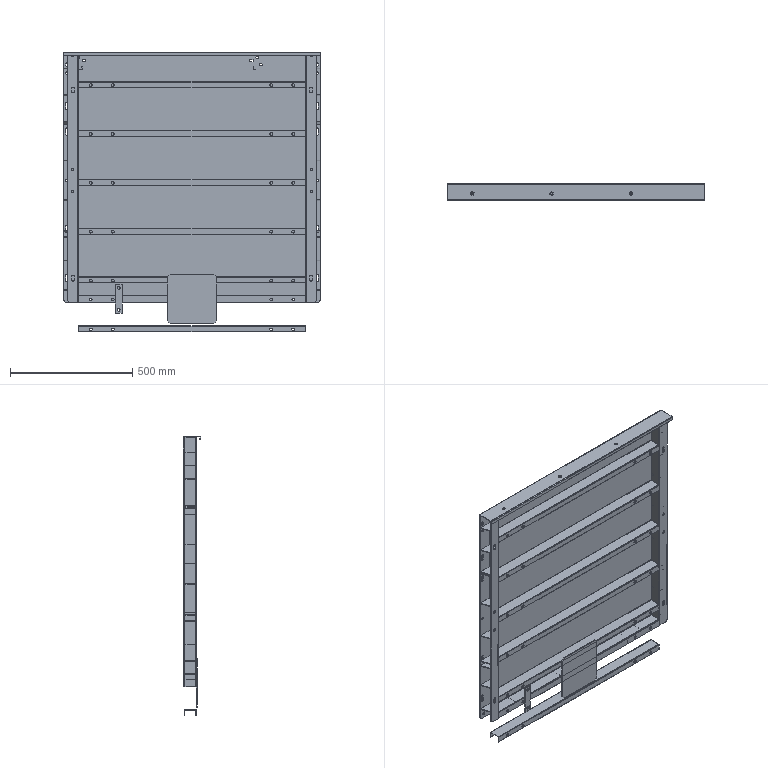Part | 43 solids | 888 faces | box 1050 x 70 x 1145 mm | volume 5959191 mm3 | plane 562 | cylinder 308 | cone 18 | commonest cylinder face diameters 11 x116 10 x90 12 x22 0.4 x20 4.4 x12 10.5 x12